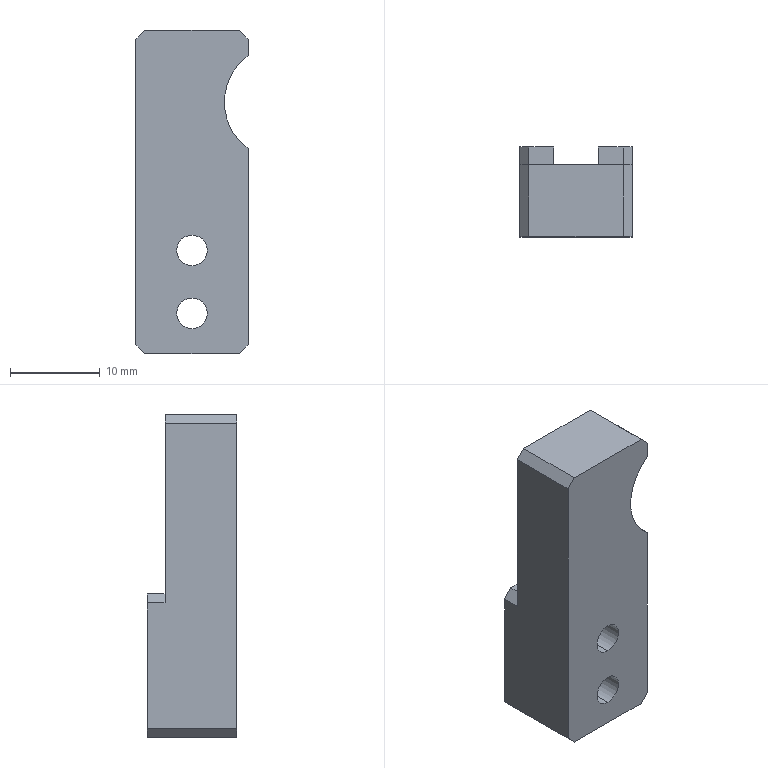Part | STEP file | PN_0015 | 1 solid | 24 faces | box 12.5 x 10 x 36 mm | volume 3520 mm3 | plane 19 | cylinder 5 | commonest cylinder face diameters 3.4 x4 12.9 x1